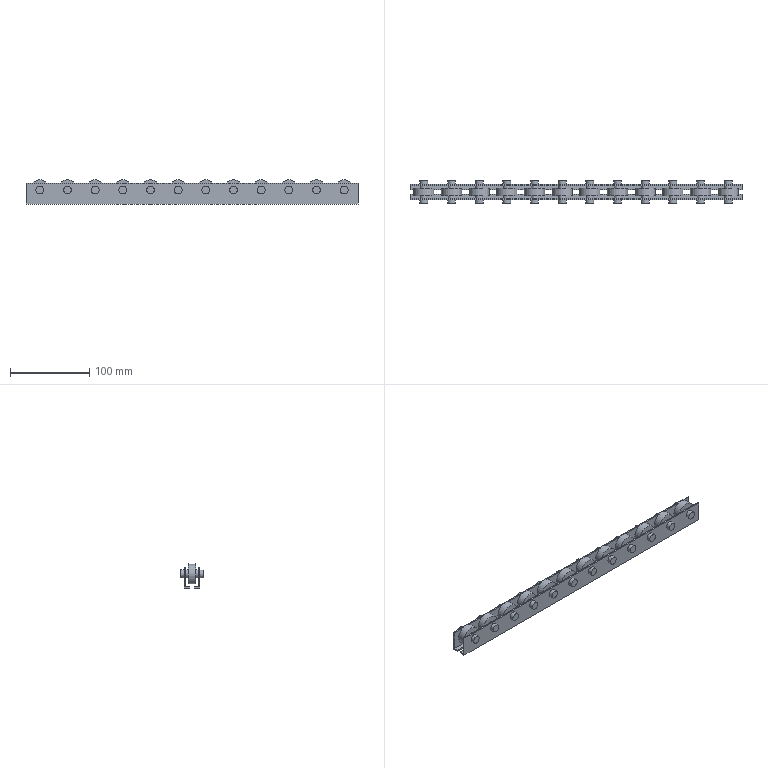Part | NX | features solid 2 | 1 solid | 124 faces | box 420 x 29 x 30.5 mm | volume 112760 mm3 | plane 64 | cylinder 60 | commonest cylinder face diameters 10 x48 25.4 x12